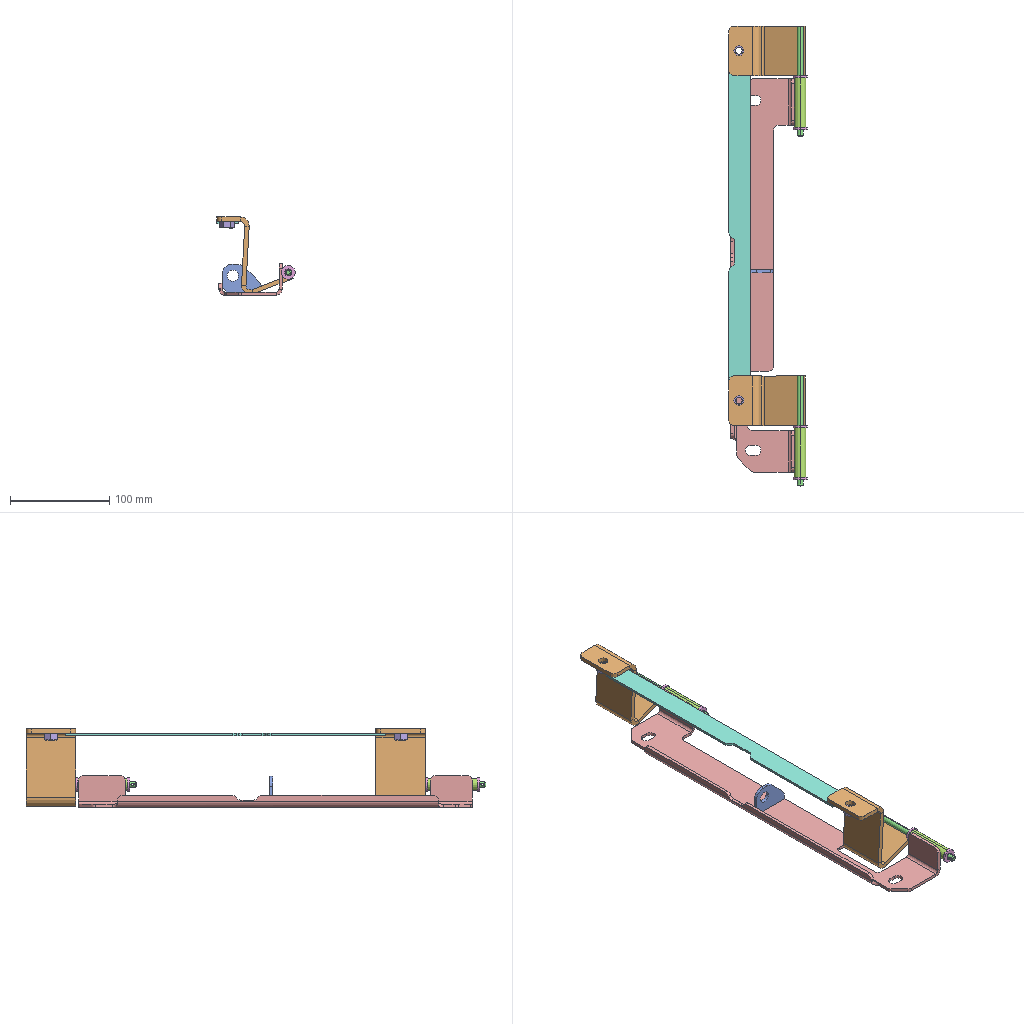Assembly | SolidWorks | 10 different items | 18 placed | box 79 x 464 x 79 mm
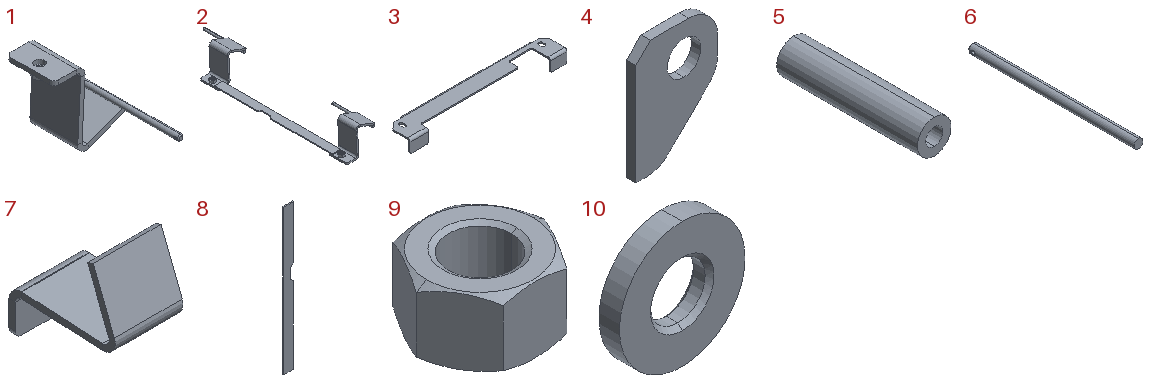Parts list (item | name | quantity | parent item | size | volume | features):
1 | (subassembly) | x2 | in 2 | 77.035 x 111 x 78.274 mm | 37259 mm3 | -
2 | (subassembly) | x1 | - | 77.035 x 464 x 78.274 mm | 90461 mm3 | features LocalLPattern 1, ReferencePattern 1
3 | - | x1 | - | 397 x 64 x 32 mm | 66915 mm3 | features ICE 2, Fillet 1, FlatPattern 1, Fold 1, SMBaseFlange 1, SheetMetal 1, UnFold 1
4 | - | x1 | - | 28 x 3.2 x 39.8 mm | 2478 mm3 | features FlatPattern 1, SMBaseFlange 1, SheetMetal 1
5 | - | x2 | - | 12 x 50 x 12 mm | 4194 mm3 | features Extrusion 1
6 | - | x2 | in 1 | 6 x 111 x 6 mm | 3110 mm3 | features ICE 2, Chamfer 1, Extrusion 1, MirrorPattern 1
7 | - | x2 | in 1 | 50 x 78.274 x 77.035 mm | 33443 mm3 | features Fillet 1, FlatPattern 1, ICE 1, SMBaseFlange 1, SheetMetal 1
8 | - | x1 | in 2 | 22 x 2.3 x 323 mm | 15944 mm3 | features Fillet 1, FlatPattern 1, SMBaseFlange 1, SheetMetal 1
9 | - | x2 | in 1 | 27.713 x 24 x 14.8 mm | 5071 mm3 | features RevCut 2, Chamfer 1, Extrusion 1, LPattern 1
10 | - | x4 | - | 14 x 2.3 x 14 mm | 281.788 mm3 | features Chamfer 1, FlatPattern 1, SMBaseFlange 1, SheetMetal 1
Mates (type | each side: item.copy, entity, surface, feature):
In the top assembly
Coincident | 3.1 face plane Base-Flange1 | 4.1 face plane Base-Flange1 | 2 times
DistanceDim | 4.1 face plane Base-Flange1 | 3.1 face plane Base-Flange1
DistanceDim | 3.1 face plane Base-Flange1 | 5.1 face cylinder Boss-Extrude1
DistanceDim | 5.1 face cylinder Boss-Extrude1 | 3.1 face plane Base-Flange1
DistanceDim | 5.1 face plane Boss-Extrude1 | 3.1 face plane Base-Flange1
Parallel | 3.1 face plane Base-Flange1 | 5.1 plane
Coincident | 5.1 face plane Boss-Extrude1 | 10.1 face plane Base-Flange1
Concentric | 5.1 face cylinder Boss-Extrude1 | 10.1 face cylinder Base-Flange1
Parallel | 10.1 plane | assembly plane
Coincident | 5.1 face plane Boss-Extrude1 | 10.2 face plane Base-Flange1
Concentric | 5.1 face cylinder Boss-Extrude1 | 10.2 face cylinder Base-Flange1
Parallel | 10.2 plane | assembly plane
Concentric | 5.1 face cylinder Boss-Extrude1 | 6.1 face cylinder Boss-Extrude1
Coincident | 10.3 face plane Base-Flange1 | 7.1 face plane Base-Flange1
In subassembly 2
Coincident | 8.1 face plane Base-Flange1 | 7.2 face plane Base-Flange1 | 2 times
DistanceDim | 8.1 face plane Base-Flange1 | 7.2 face plane Base-Flange1
In subassembly 1
Concentric | 7.3 face cylinder Cut-Extrude1 | 9.1 face cone EndChamfer
Coincident | 7.3 face plane Base-Flange1 | 9.1 face plane BaseNut
Parallel | 7.3 face plane Base-Flange1 | 9.1 face plane BaseNut
DistanceDim | 7.3 face plane Base-Flange1 | 6.2 face cylinder Boss-Extrude1 | 2 times
Parallel | 7.3 face plane Base-Flange1 | 6.2 plane
Coincident | 7.3 face plane Base-Flange1 | 6.2 face plane Boss-Extrude1